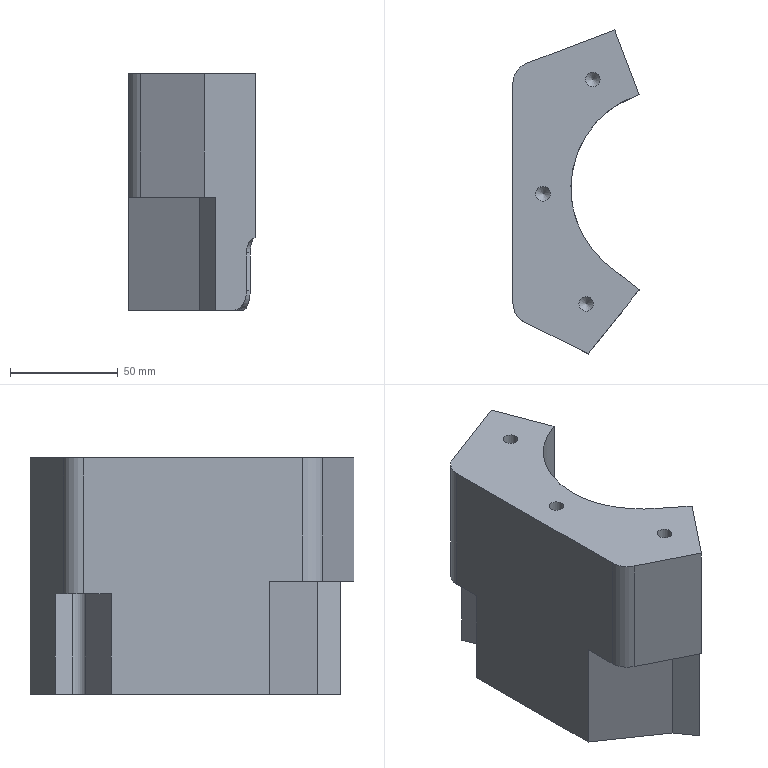Part | NX | features 8 2 | 1 solid | 38 faces | box 58.524 x 150.094 x 109.5 mm | volume 519516 mm3 | plane 15 | cylinder 13 | cone 5 | spline 4 | torus 1 | commonest cylinder face diameters 6.8 x3 8.5 x2 14 x2 18 x2 20 x2 10 x1
STEP:
#1=CARTESIAN_POINT('',(1901.4,-118.,66.));
#2=VERTEX_POINT('',#1);
#3=CARTESIAN_POINT('',(1898.,-118.,66.));
#4=DIRECTION('',(0.,0.,1.));
#5=DIRECTION('',(1.,0.,0.));
#6=AXIS2_PLACEMENT_3D('',#3,#4,#5);
#7=CIRCLE('',#6,3.4);
#8=EDGE_CURVE('',#2,#2,#7,.T.);
#9=ORIENTED_EDGE('',*,*,#8,.F.);
#10=EDGE_LOOP('',(#9));
#11=FACE_BOUND('',#10,.T.);
#12=CARTESIAN_POINT('',(1884.,-66.828,66.));
#13=VERTEX_POINT('',#12);
#14=CARTESIAN_POINT('',(1884.,-168.522,66.));
#15=VERTEX_POINT('',#14);
#16=CARTESIAN_POINT('',(1884.,-218.467,66.));
#17=DIRECTION('',(0.,-1.,0.));
#18=VECTOR('',#17,1000.);
#19=LINE('',#16,#18);
#20=EDGE_CURVE('',#13,#15,#19,.T.);
#21=ORIENTED_EDGE('',*,*,#20,.T.);
#22=CARTESIAN_POINT('',(1889.537,-177.471,66.));
#23=VERTEX_POINT('',#22);
#24=CARTESIAN_POINT('',(1894.,-168.522,66.));
#25=DIRECTION('',(0.,0.,1.));
#26=DIRECTION('',(1.,0.,0.));
#27=AXIS2_PLACEMENT_3D('',#24,#25,#26);
#28=CIRCLE('',#27,10.);
#29=EDGE_CURVE('',#15,#23,#28,.T.);
#30=ORIENTED_EDGE('',*,*,#29,.T.);
#31=CARTESIAN_POINT('',(1918.94,-192.136,66.));
#32=VERTEX_POINT('',#31);
#33=CARTESIAN_POINT('',(2033.826,-249.437,66.));
#34=DIRECTION('',(0.8949,-0.4463,0.));
#35=VECTOR('',#34,1000.);
#36=LINE('',#33,#35);
#37=EDGE_CURVE('',#23,#32,#36,.T.);
#38=ORIENTED_EDGE('',*,*,#37,.T.);
#39=CARTESIAN_POINT('',(1942.524,-162.487,66.));
#40=VERTEX_POINT('',#39);
#41=CARTESIAN_POINT('',(1956.62,-144.766,66.));
#42=DIRECTION('',(0.6225,0.7826,0.));
#43=VECTOR('',#42,1000.);
#44=LINE('',#41,#43);
#45=EDGE_CURVE('',#32,#40,#44,.T.);
#46=ORIENTED_EDGE('',*,*,#45,.T.);
#47=CARTESIAN_POINT('',(1942.524,-71.965,66.));
#48=VERTEX_POINT('',#47);
#49=CARTESIAN_POINT('',(1942.524,-71.965,66.));
#50=CARTESIAN_POINT('',(1940.246,-72.828,66.));
#51=CARTESIAN_POINT('',(1935.71,-74.591,66.));
#52=CARTESIAN_POINT('',(1929.54,-78.399,66.));
#53=CARTESIAN_POINT('',(1923.928,-83.204,66.));
#54=CARTESIAN_POINT('',(1919.28,-88.703,66.));
#55=CARTESIAN_POINT('',(1915.465,-95.025,66.));
#56=CARTESIAN_POINT('',(1912.762,-101.765,66.));
#57=CARTESIAN_POINT('',(1911.14,-108.951,66.));
#58=CARTESIAN_POINT('',(1910.547,-118.647,66.));
#59=CARTESIAN_POINT('',(1912.303,-128.367,66.));
#60=CARTESIAN_POINT('',(1916.274,-137.266,66.));
#61=CARTESIAN_POINT('',(1920.299,-143.399,66.));
#62=CARTESIAN_POINT('',(1925.194,-148.787,66.));
#63=CARTESIAN_POINT('',(1932.973,-154.837,66.));
#64=CARTESIAN_POINT('',(1938.688,-159.435,66.));
#65=CARTESIAN_POINT('',(1942.524,-162.487,66.));
#66=B_SPLINE_CURVE_WITH_KNOTS('',3,(#49,#50,#51,#52,#53,#54,#55,#56,#57,#58,#59,#60,#61,#62,#63,#64,#65),.UNSPECIFIED.,.F.,.F.,(4,1,1,1,1,1,1,1,1,1,1,1,1,1,4),(0.,0.007238,0.01448,0.02172,0.02895,0.03619,0.04343,0.05067,0.05791,0.07238,0.07962,0.08686,0.0941,0.1013,0.1158),.UNSPECIFIED.);
#67=EDGE_CURVE('',#48,#40,#66,.T.);
#68=ORIENTED_EDGE('',*,*,#67,.F.);
#69=CARTESIAN_POINT('',(1931.184,-42.042,66.));
#70=VERTEX_POINT('',#69);
#71=CARTESIAN_POINT('',(2004.479,-235.443,66.));
#72=DIRECTION('',(-0.3544,0.9351,0.));
#73=VECTOR('',#72,1000.);
#74=LINE('',#71,#73);
#75=EDGE_CURVE('',#48,#70,#74,.T.);
#76=ORIENTED_EDGE('',*,*,#75,.T.);
#77=CARTESIAN_POINT('',(1890.456,-57.477,66.));
#78=VERTEX_POINT('',#77);
#79=CARTESIAN_POINT('',(1990.095,-19.716,66.));
#80=DIRECTION('',(0.9351,0.3544,0.));
#81=VECTOR('',#80,1000.);
#82=LINE('',#79,#81);
#83=EDGE_CURVE('',#78,#70,#82,.T.);
#84=ORIENTED_EDGE('',*,*,#83,.F.);
#85=CARTESIAN_POINT('',(1894.,-66.828,66.));
#86=DIRECTION('',(0.,0.,1.));
#87=DIRECTION('',(1.,0.,0.));
#88=AXIS2_PLACEMENT_3D('',#85,#86,#87);
#89=CIRCLE('',#88,10.);
#90=EDGE_CURVE('',#78,#13,#89,.T.);
#91=ORIENTED_EDGE('',*,*,#90,.T.);
#92=EDGE_LOOP('',(#21,#30,#38,#46,#68,#76,#84,#91));
#93=FACE_BOUND('',#92,.T.);
#94=CARTESIAN_POINT('',(1921.4,-169.,66.));
#95=VERTEX_POINT('',#94);
#96=CARTESIAN_POINT('',(1918.,-169.,66.));
#97=DIRECTION('',(0.,0.,1.));
#98=DIRECTION('',(1.,0.,0.));
#99=AXIS2_PLACEMENT_3D('',#96,#97,#98);
#100=CIRCLE('',#99,3.4);
#101=EDGE_CURVE('',#95,#95,#100,.T.);
#102=ORIENTED_EDGE('',*,*,#101,.F.);
#103=EDGE_LOOP('',(#102));
#104=FACE_BOUND('',#103,.T.);
#105=CARTESIAN_POINT('',(1924.4,-65.,66.));
#106=VERTEX_POINT('',#105);
#107=CARTESIAN_POINT('',(1921.,-65.,66.));
#108=DIRECTION('',(0.,0.,1.));
#109=DIRECTION('',(1.,0.,0.));
#110=AXIS2_PLACEMENT_3D('',#107,#108,#109);
#111=CIRCLE('',#110,3.4);
#112=EDGE_CURVE('',#106,#106,#111,.T.);
#113=ORIENTED_EDGE('',*,*,#112,.F.);
#114=EDGE_LOOP('',(#113));
#115=FACE_BOUND('',#114,.T.);
#116=CARTESIAN_POINT('',(2049.273,-218.467,66.));
#117=DIRECTION('',(0.,0.,1.));
#118=DIRECTION('',(-1.,0.,0.));
#119=AXIS2_PLACEMENT_3D('',#116,#117,#118);
#120=PLANE('',#119);
#121=ADVANCED_FACE('',(#11,#93,#104,#115),#120,.T.);
#122=CARTESIAN_POINT('',(1884.,-79.693,3.));
#123=VERTEX_POINT('',#122);
#124=CARTESIAN_POINT('',(1884.,-66.828,3.));
#125=VERTEX_POINT('',#124);
#126=CARTESIAN_POINT('',(1884.,-36.,3.));
#127=DIRECTION('',(0.,1.,0.));
#128=VECTOR('',#127,1000.);
#129=LINE('',#126,#128);
#130=EDGE_CURVE('',#123,#125,#129,.T.);
#131=ORIENTED_EDGE('',*,*,#130,.T.);
#132=CARTESIAN_POINT('',(1890.456,-57.477,3.));
#133=VERTEX_POINT('',#132);
#134=CARTESIAN_POINT('',(1894.,-66.828,3.));
#135=DIRECTION('',(0.,0.,-1.));
#136=DIRECTION('',(1.,0.,0.));
#137=AXIS2_PLACEMENT_3D('',#134,#135,#136);
#138=CIRCLE('',#137,10.);
#139=EDGE_CURVE('',#125,#133,#138,.T.);
#140=ORIENTED_EDGE('',*,*,#139,.T.);
#141=CARTESIAN_POINT('',(1900.443,-53.692,3.));
#142=VERTEX_POINT('',#141);
#143=CARTESIAN_POINT('',(1990.095,-19.716,3.));
#144=DIRECTION('',(0.9351,0.3544,0.));
#145=VECTOR('',#144,1000.);
#146=LINE('',#143,#145);
#147=EDGE_CURVE('',#133,#142,#146,.T.);
#148=ORIENTED_EDGE('',*,*,#147,.T.);
#149=CARTESIAN_POINT('',(1903.559,-61.916,3.));
#150=VERTEX_POINT('',#149);
#151=CARTESIAN_POINT('',(1902.952,-60.314,3.));
#152=DIRECTION('',(-0.3544,0.9351,0.));
#153=VECTOR('',#152,1000.);
#154=LINE('',#151,#153);
#155=EDGE_CURVE('',#150,#142,#154,.T.);
#156=ORIENTED_EDGE('',*,*,#155,.F.);
#157=CARTESIAN_POINT('',(1901.669,-67.84,3.));
#158=VERTEX_POINT('',#157);
#159=CARTESIAN_POINT('',(1898.884,-63.688,3.));
#160=DIRECTION('',(0.,0.,-1.));
#161=DIRECTION('',(1.,0.,0.));
#162=AXIS2_PLACEMENT_3D('',#159,#160,#161);
#163=CIRCLE('',#162,5.);
#164=EDGE_CURVE('',#150,#158,#163,.T.);
#165=ORIENTED_EDGE('',*,*,#164,.T.);
#166=CARTESIAN_POINT('',(1894.226,-72.833,3.));
#167=DIRECTION('',(0.8305,0.5571,0.));
#168=VECTOR('',#167,1000.);
#169=LINE('',#166,#168);
#170=EDGE_CURVE('',#123,#158,#169,.T.);
#171=ORIENTED_EDGE('',*,*,#170,.F.);
#172=EDGE_LOOP('',(#131,#140,#148,#156,#165,#171));
#173=FACE_BOUND('',#172,.T.);
#174=CARTESIAN_POINT('',(1899.25,-66.,3.));
#175=VERTEX_POINT('',#174);
#176=CARTESIAN_POINT('',(1895.,-66.,3.));
#177=DIRECTION('',(0.,0.,-1.));
#178=DIRECTION('',(1.,0.,0.));
#179=AXIS2_PLACEMENT_3D('',#176,#177,#178);
#180=CIRCLE('',#179,4.25);
#181=EDGE_CURVE('',#175,#175,#180,.T.);
#182=ORIENTED_EDGE('',*,*,#181,.F.);
#183=EDGE_LOOP('',(#182));
#184=FACE_BOUND('',#183,.T.);
#185=CARTESIAN_POINT('',(1890.975,-67.988,3.));
#186=DIRECTION('',(0.,0.,1.));
#187=DIRECTION('',(-1.,0.,0.));
#188=AXIS2_PLACEMENT_3D('',#185,#186,#187);
#189=PLANE('',#188);
#190=ADVANCED_FACE('',(#173,#184),#189,.F.);
#191=CARTESIAN_POINT('',(1884.,-79.693,-43.5));
#192=VERTEX_POINT('',#191);
#193=CARTESIAN_POINT('',(1884.,-79.693,0.));
#194=DIRECTION('',(0.,0.,1.));
#195=VECTOR('',#194,1000.);
#196=LINE('',#193,#195);
#197=EDGE_CURVE('',#192,#123,#196,.T.);
#198=ORIENTED_EDGE('',*,*,#197,.F.);
#199=CARTESIAN_POINT('',(1884.,-152.801,-43.5));
#200=VERTEX_POINT('',#199);
#201=CARTESIAN_POINT('',(1884.,-66.746,-43.5));
#202=DIRECTION('',(0.,1.,0.000000004));
#203=VECTOR('',#202,1000.);
#204=LINE('',#201,#203);
#205=EDGE_CURVE('',#200,#192,#204,.T.);
#206=ORIENTED_EDGE('',*,*,#205,.F.);
#207=CARTESIAN_POINT('',(1884.,-152.801,8.9));
#208=VERTEX_POINT('',#207);
#209=CARTESIAN_POINT('',(1884.,-152.801,0.));
#210=DIRECTION('',(0.,0.,-1.));
#211=VECTOR('',#210,1000.);
#212=LINE('',#209,#211);
#213=EDGE_CURVE('',#208,#200,#212,.T.);
#214=ORIENTED_EDGE('',*,*,#213,.F.);
#215=CARTESIAN_POINT('',(1884.,-168.522,8.9));
#216=VERTEX_POINT('',#215);
#217=CARTESIAN_POINT('',(1884.,-36.,8.9));
#218=DIRECTION('',(0.,1.,0.));
#219=VECTOR('',#218,1000.);
#220=LINE('',#217,#219);
#221=EDGE_CURVE('',#216,#208,#220,.T.);
#222=ORIENTED_EDGE('',*,*,#221,.F.);
#223=CARTESIAN_POINT('',(1884.,-168.522,0.));
#224=DIRECTION('',(0.,0.,1.));
#225=VECTOR('',#224,1000.);
#226=LINE('',#223,#225);
#227=EDGE_CURVE('',#216,#15,#226,.T.);
#228=ORIENTED_EDGE('',*,*,#227,.T.);
#229=ORIENTED_EDGE('',*,*,#20,.F.);
#230=CARTESIAN_POINT('',(1884.,-66.828,0.));
#231=DIRECTION('',(0.,0.,-1.));
#232=VECTOR('',#231,1000.);
#233=LINE('',#230,#232);
#234=EDGE_CURVE('',#13,#125,#233,.T.);
#235=ORIENTED_EDGE('',*,*,#234,.T.);
#236=ORIENTED_EDGE('',*,*,#130,.F.);
#237=EDGE_LOOP('',(#198,#206,#214,#222,#228,#229,#235,#236));
#238=FACE_BOUND('',#237,.T.);
#239=CARTESIAN_POINT('',(1884.,-36.,0.));
#240=DIRECTION('',(-1.,0.,0.));
#241=DIRECTION('',(0.,0.,-1.));
#242=AXIS2_PLACEMENT_3D('',#239,#240,#241);
#243=PLANE('',#242);
#244=ADVANCED_FACE('',(#238),#243,.T.);
#245=ORIENTED_EDGE('',*,*,#37,.F.);
#246=CARTESIAN_POINT('',(1889.537,-177.471,8.9));
#247=VERTEX_POINT('',#246);
#248=CARTESIAN_POINT('',(1889.537,-177.471,-27.5));
#249=DIRECTION('',(0.,0.,-1.));
#250=VECTOR('',#249,1000.);
#251=LINE('',#248,#250);
#252=EDGE_CURVE('',#23,#247,#251,.T.);
#253=ORIENTED_EDGE('',*,*,#252,.T.);
#254=CARTESIAN_POINT('',(1918.94,-192.136,8.9));
#255=VERTEX_POINT('',#254);
#256=CARTESIAN_POINT('',(1975.42,-220.307,8.9));
#257=DIRECTION('',(-0.8949,0.4463,0.));
#258=VECTOR('',#257,1000.);
#259=LINE('',#256,#258);
#260=EDGE_CURVE('',#255,#247,#259,.T.);
#261=ORIENTED_EDGE('',*,*,#260,.F.);
#262=CARTESIAN_POINT('',(1918.94,-192.136,-116.522));
#263=DIRECTION('',(0.,0.,-1.));
#264=VECTOR('',#263,1000.);
#265=LINE('',#262,#264);
#266=EDGE_CURVE('',#32,#255,#265,.T.);
#267=ORIENTED_EDGE('',*,*,#266,.F.);
#268=EDGE_LOOP('',(#245,#253,#261,#267));
#269=FACE_BOUND('',#268,.T.);
#270=CARTESIAN_POINT('',(1975.42,-220.307,-27.5));
#271=DIRECTION('',(-0.4463,-0.8949,0.));
#272=DIRECTION('',(-0.8949,0.4463,0.));
#273=AXIS2_PLACEMENT_3D('',#270,#271,#272);
#274=PLANE('',#273);
#275=ADVANCED_FACE('',(#269),#274,.T.);
#276=CARTESIAN_POINT('',(1924.001,-185.773,8.9));
#277=VERTEX_POINT('',#276);
#278=CARTESIAN_POINT('',(1885.875,-233.704,8.9));
#279=DIRECTION('',(-0.6225,-0.7826,0.));
#280=VECTOR('',#279,1000.);
#281=LINE('',#278,#280);
#282=EDGE_CURVE('',#277,#255,#281,.T.);
#283=ORIENTED_EDGE('',*,*,#282,.F.);
#284=CARTESIAN_POINT('',(1924.001,-185.773,-43.5));
#285=VERTEX_POINT('',#284);
#286=CARTESIAN_POINT('',(1924.001,-185.773,-116.522));
#287=DIRECTION('',(0.,0.,-1.));
#288=VECTOR('',#287,1000.);
#289=LINE('',#286,#288);
#290=EDGE_CURVE('',#277,#285,#289,.T.);
#291=ORIENTED_EDGE('',*,*,#290,.T.);
#292=CARTESIAN_POINT('',(1932.875,-174.617,-43.5));
#293=VERTEX_POINT('',#292);
#294=CARTESIAN_POINT('',(1938.478,-167.574,-43.5));
#295=DIRECTION('',(-0.6225,-0.7826,-0.000000003));
#296=VECTOR('',#295,1000.);
#297=LINE('',#294,#296);
#298=EDGE_CURVE('',#293,#285,#297,.T.);
#299=ORIENTED_EDGE('',*,*,#298,.F.);
#300=CARTESIAN_POINT('',(1938.478,-167.574,-34.5));
#301=VERTEX_POINT('',#300);
#302=CARTESIAN_POINT('',(1932.875,-174.617,-34.5));
#303=DIRECTION('',(0.7826,-0.6225,0.));
#304=DIRECTION('',(0.6225,0.7826,0.));
#305=AXIS2_PLACEMENT_3D('',#302,#303,#304);
#306=CIRCLE('',#305,9.);
#307=EDGE_CURVE('',#293,#301,#306,.T.);
#308=ORIENTED_EDGE('',*,*,#307,.T.);
#309=CARTESIAN_POINT('',(1938.478,-167.574,-17.));
#310=VERTEX_POINT('',#309);
#311=CARTESIAN_POINT('',(1938.478,-167.574,-0.00000039));
#312=DIRECTION('',(-0.000000002,-0.000000002,1.));
#313=VECTOR('',#312,1000.);
#314=LINE('',#311,#313);
#315=EDGE_CURVE('',#301,#310,#314,.T.);
#316=ORIENTED_EDGE('',*,*,#315,.T.);
#317=CARTESIAN_POINT('',(1942.524,-162.487,-10.018));
#318=VERTEX_POINT('',#317);
#319=CARTESIAN_POINT('',(1942.835,-162.095,-17.));
#320=DIRECTION('',(-0.7826,0.6225,0.));
#321=DIRECTION('',(0.6225,0.7826,0.));
#322=AXIS2_PLACEMENT_3D('',#319,#320,#321);
#323=CIRCLE('',#322,7.);
#324=EDGE_CURVE('',#310,#318,#323,.T.);
#325=ORIENTED_EDGE('',*,*,#324,.T.);
#326=CARTESIAN_POINT('',(1942.524,-162.487,7.385));
#327=DIRECTION('',(0.,0.,-1.));
#328=VECTOR('',#327,1000.);
#329=LINE('',#326,#328);
#330=EDGE_CURVE('',#40,#318,#329,.T.);
#331=ORIENTED_EDGE('',*,*,#330,.F.);
#332=ORIENTED_EDGE('',*,*,#45,.F.);
#333=ORIENTED_EDGE('',*,*,#266,.T.);
#334=EDGE_LOOP('',(#283,#291,#299,#308,#316,#325,#331,#332,#333));
#335=FACE_BOUND('',#334,.T.);
#336=CARTESIAN_POINT('',(1885.875,-233.704,-116.522));
#337=DIRECTION('',(0.7826,-0.6225,0.));
#338=DIRECTION('',(-0.6225,-0.7826,0.));
#339=AXIS2_PLACEMENT_3D('',#336,#337,#338);
#340=PLANE('',#339);
#341=ADVANCED_FACE('',(#335),#340,.T.);
#342=ORIENTED_EDGE('',*,*,#298,.T.);
#343=CARTESIAN_POINT('',(1916.658,-175.233,-43.5));
#344=VERTEX_POINT('',#343);
#345=CARTESIAN_POINT('',(1872.732,-112.188,-43.5));
#346=DIRECTION('',(-0.5717,0.8205,0.000000004));
#347=VECTOR('',#346,1000.);
#348=LINE('',#345,#347);
#349=EDGE_CURVE('',#285,#344,#348,.T.);
#350=ORIENTED_EDGE('',*,*,#349,.T.);
#351=CARTESIAN_POINT('',(1880.497,-150.395,-43.5));
#352=DIRECTION('',(0.8243,-0.5662,-0.000000003));
#353=VECTOR('',#352,1000.);
#354=LINE('',#351,#353);
#355=EDGE_CURVE('',#200,#344,#354,.T.);
#356=ORIENTED_EDGE('',*,*,#355,.F.);
#357=ORIENTED_EDGE('',*,*,#205,.T.);
#358=CARTESIAN_POINT('',(1901.669,-67.84,-43.5));
#359=VERTEX_POINT('',#358);
#360=CARTESIAN_POINT('',(1927.2,-50.714,-43.5));
#361=DIRECTION('',(-0.8305,-0.5571,-0.000000002));
#362=VECTOR('',#361,1000.);
#363=LINE('',#360,#362);
#364=EDGE_CURVE('',#359,#192,#363,.T.);
#365=ORIENTED_EDGE('',*,*,#364,.F.);
#366=CARTESIAN_POINT('',(1903.559,-61.916,-43.5));
#367=VERTEX_POINT('',#366);
#368=CARTESIAN_POINT('',(1898.884,-63.688,-43.5));
#369=DIRECTION('',(0.000000001,-0.000000004,1.));
#370=DIRECTION('',(0.,1.,0.000000004));
#371=AXIS2_PLACEMENT_3D('',#368,#369,#370);
#372=CIRCLE('',#371,5.);
#373=EDGE_CURVE('',#359,#367,#372,.T.);
#374=ORIENTED_EDGE('',*,*,#373,.T.);
#375=CARTESIAN_POINT('',(1900.443,-53.692,-43.5));
#376=VERTEX_POINT('',#375);
#377=CARTESIAN_POINT('',(1909.48,-77.537,-43.5));
#378=DIRECTION('',(0.3544,-0.9351,-0.000000004));
#379=VECTOR('',#378,1000.);
#380=LINE('',#377,#379);
#381=EDGE_CURVE('',#376,#367,#380,.T.);
#382=ORIENTED_EDGE('',*,*,#381,.F.);
#383=CARTESIAN_POINT('',(1931.184,-42.042,-43.5));
#384=VERTEX_POINT('',#383);
#385=CARTESIAN_POINT('',(1990.095,-19.716,-43.5));
#386=DIRECTION('',(-0.9351,-0.3544,-0.000000001));
#387=VECTOR('',#386,1000.);
#388=LINE('',#385,#387);
#389=EDGE_CURVE('',#384,#376,#388,.T.);
#390=ORIENTED_EDGE('',*,*,#389,.F.);
#391=CARTESIAN_POINT('',(1937.031,-57.471,-43.5));
#392=VERTEX_POINT('',#391);
#393=CARTESIAN_POINT('',(1940.221,-65.887,-43.5));
#394=DIRECTION('',(-0.3544,0.9351,0.000000004));
#395=VECTOR('',#394,1000.);
#396=LINE('',#393,#395);
#397=EDGE_CURVE('',#392,#384,#396,.T.);
#398=ORIENTED_EDGE('',*,*,#397,.F.);
#399=CARTESIAN_POINT('',(1934.761,-58.331,-43.5));
#400=VERTEX_POINT('',#399);
#401=CARTESIAN_POINT('',(1937.031,-57.471,-43.5));
#402=CARTESIAN_POINT('',(1936.275,-57.758,-43.5));
#403=CARTESIAN_POINT('',(1935.518,-58.045,-43.5));
#404=CARTESIAN_POINT('',(1934.761,-58.331,-43.5));
#405=B_SPLINE_CURVE_WITH_KNOTS('',3,(#401,#402,#403,#404),.UNSPECIFIED.,.F.,.F.,(4,4),(0.,1.),.PIECEWISE_BEZIER_KNOTS.);
#406=EDGE_CURVE('',#392,#400,#405,.T.);
#407=ORIENTED_EDGE('',*,*,#406,.T.);
#408=CARTESIAN_POINT('',(1918.407,-163.108,-43.5));
#409=VERTEX_POINT('',#408);
#410=CARTESIAN_POINT('',(1934.761,-58.331,-43.5));
#411=CARTESIAN_POINT('',(1933.539,-58.796,-43.5));
#412=CARTESIAN_POINT('',(1931.034,-59.837,-43.5));
#413=CARTESIAN_POINT('',(1926.249,-62.216,-43.5));
#414=CARTESIAN_POINT('',(1918.279,-67.207,-43.5));
#415=CARTESIAN_POINT('',(1908.459,-76.481,-43.5));
#416=CARTESIAN_POINT('',(1900.024,-90.316,-43.5));
#417=CARTESIAN_POINT('',(1895.397,-105.855,-43.5));
#418=CARTESIAN_POINT('',(1895.063,-122.038,-43.5));
#419=CARTESIAN_POINT('',(1898.885,-137.806,-43.5));
#420=CARTESIAN_POINT('',(1905.421,-149.636,-43.5));
#421=CARTESIAN_POINT('',(1911.469,-156.801,-43.5));
#422=CARTESIAN_POINT('',(1915.332,-160.551,-43.5));
#423=CARTESIAN_POINT('',(1917.34,-162.258,-43.5));
#424=CARTESIAN_POINT('',(1918.407,-163.108,-43.5));
#425=B_SPLINE_CURVE_WITH_KNOTS('',3,(#410,#411,#412,#413,#414,#415,#416,#417,#418,#419,#420,#421,#422,#423,#424),.UNSPECIFIED.,.F.,.F.,(4,1,1,1,1,1,1,1,1,1,1,1,4),(0.,0.03125,0.0625,0.125,0.25,0.375,0.5,0.625,0.75,0.875,0.9375,0.9688,1.),.UNSPECIFIED.);
#426=EDGE_CURVE('',#400,#409,#425,.T.);
#427=ORIENTED_EDGE('',*,*,#426,.T.);
#428=CARTESIAN_POINT('',(1918.407,-163.108,-43.5));
#429=CARTESIAN_POINT('',(1923.229,-166.944,-43.5));
#430=CARTESIAN_POINT('',(1928.052,-170.781,-43.5));
#431=CARTESIAN_POINT('',(1932.875,-174.617,-43.5));
#432=B_SPLINE_CURVE_WITH_KNOTS('',3,(#428,#429,#430,#431),.UNSPECIFIED.,.F.,.F.,(4,4),(0.,1.),.PIECEWISE_BEZIER_KNOTS.);
#433=EDGE_CURVE('',#409,#293,#432,.T.);
#434=ORIENTED_EDGE('',*,*,#433,.T.);
#435=EDGE_LOOP('',(#342,#350,#356,#357,#365,#374,#382,#390,#398,#407,#427,#434));
#436=FACE_BOUND('',#435,.T.);
#437=CARTESIAN_POINT('',(1937.954,-66.746,-43.5));
#438=DIRECTION('',(-0.000000001,0.000000004,-1.));
#439=DIRECTION('',(0.3552,-0.9348,-0.000000004));
#440=AXIS2_PLACEMENT_3D('',#437,#438,#439);
#441=PLANE('',#440);
#442=ADVANCED_FACE('',(#436),#441,.T.);
#443=CARTESIAN_POINT('',(1940.221,-65.887,-34.5));
#444=VERTEX_POINT('',#443);
#445=CARTESIAN_POINT('',(1937.031,-57.471,-34.5));
#446=DIRECTION('',(0.9351,0.3544,0.));
#447=DIRECTION('',(-0.3544,0.9351,0.));
#448=AXIS2_PLACEMENT_3D('',#445,#446,#447);
#449=CIRCLE('',#448,9.);
#450=EDGE_CURVE('',#444,#392,#449,.T.);
#451=ORIENTED_EDGE('',*,*,#450,.F.);
#452=CARTESIAN_POINT('',(1937.954,-66.746,-34.5));
#453=VERTEX_POINT('',#452);
#454=CARTESIAN_POINT('',(1959.053,-58.75,-34.5));
#455=DIRECTION('',(-0.9351,-0.3544,-0.000000001));
#456=VECTOR('',#455,1000.);
#457=LINE('',#454,#456);
#458=EDGE_CURVE('',#444,#453,#457,.T.);
#459=ORIENTED_EDGE('',*,*,#458,.T.);
#460=CARTESIAN_POINT('',(1934.765,-58.33,-34.5));
#461=DIRECTION('',(-0.9351,-0.3544,-0.000000001));
#462=DIRECTION('',(-0.3544,0.9351,0.000000003));
#463=AXIS2_PLACEMENT_3D('',#460,#461,#462);
#464=CIRCLE('',#463,9.);
#465=EDGE_CURVE('',#400,#453,#464,.T.);
#466=ORIENTED_EDGE('',*,*,#465,.F.);
#467=ORIENTED_EDGE('',*,*,#406,.F.);
#468=EDGE_LOOP('',(#451,#459,#466,#467));
#469=FACE_BOUND('',#468,.T.);
#470=CARTESIAN_POINT('',(1977.312,-42.205,-34.5));
#471=DIRECTION('',(-0.9351,-0.3544,-0.000000001));
#472=DIRECTION('',(-0.3544,0.9351,0.));
#473=AXIS2_PLACEMENT_3D('',#470,#471,#472);
#474=CYLINDRICAL_SURFACE('',#473,9.);
#475=ADVANCED_FACE('',(#469),#474,.T.);
#476=CARTESIAN_POINT('',(1940.221,-65.887,-17.));
#477=VERTEX_POINT('',#476);
#478=CARTESIAN_POINT('',(1940.221,-65.887,0.000000056));
#479=DIRECTION('',(-0.000000001,0.000000004,-1.));
#480=VECTOR('',#479,1000.);
#481=LINE('',#478,#480);
#482=EDGE_CURVE('',#477,#444,#481,.T.);
#483=ORIENTED_EDGE('',*,*,#482,.F.);
#484=CARTESIAN_POINT('',(1937.954,-66.746,-17.));
#485=VERTEX_POINT('',#484);
#486=CARTESIAN_POINT('',(1960.935,-58.037,-17.));
#487=DIRECTION('',(-0.9351,-0.3544,-0.000000001));
#488=VECTOR('',#487,1000.);
#489=LINE('',#486,#488);
#490=EDGE_CURVE('',#477,#485,#489,.T.);
#491=ORIENTED_EDGE('',*,*,#490,.T.);
#492=CARTESIAN_POINT('',(1937.954,-66.746,-22.75));
#493=DIRECTION('',(0.000000001,-0.000000004,1.));
#494=VECTOR('',#493,1000.);
#495=LINE('',#492,#494);
#496=EDGE_CURVE('',#453,#485,#495,.T.);
#497=ORIENTED_EDGE('',*,*,#496,.F.);
#498=ORIENTED_EDGE('',*,*,#458,.F.);
#499=EDGE_LOOP('',(#483,#491,#497,#498));
#500=FACE_BOUND('',#499,.T.);
#501=CARTESIAN_POINT('',(2038.436,-28.665,0.000000056));
#502=DIRECTION('',(-0.3544,0.9351,0.000000004));
#503=DIRECTION('',(0.9351,0.3544,0.000000001));
#504=AXIS2_PLACEMENT_3D('',#501,#502,#503);
#505=PLANE('',#504);
#506=ADVANCED_FACE('',(#500),#505,.F.);
#507=CARTESIAN_POINT('',(1937.948,-66.748,-34.5));
#508=VERTEX_POINT('',#507);
#509=CARTESIAN_POINT('',(1937.948,-66.748,-34.5));
#510=CARTESIAN_POINT('',(1937.948,-66.748,-35.561));
#511=CARTESIAN_POINT('',(1937.812,-66.389,-37.852));
#512=CARTESIAN_POINT('',(1937.081,-64.461,-41.054));
#513=CARTESIAN_POINT('',(1935.946,-61.467,-43.116));
#514=CARTESIAN_POINT('',(1935.133,-59.325,-43.5));
#515=CARTESIAN_POINT('',(1934.757,-58.333,-43.5));
#516=B_SPLINE_CURVE_WITH_KNOTS('',3,(#509,#510,#511,#512,#513,#514,#515),.UNSPECIFIED.,.F.,.F.,(4,1,1,1,4),(0.,0.25,0.5,0.75,1.),.UNSPECIFIED.);
#517=EDGE_CURVE('',#400,#508,#516,.F.);
#518=ORIENTED_EDGE('',*,*,#517,.F.);
#519=ORIENTED_EDGE('',*,*,#465,.T.);
#520=CARTESIAN_POINT('',(1937.954,-66.746,-34.5));
#521=CARTESIAN_POINT('',(1937.952,-66.747,-34.5));
#522=CARTESIAN_POINT('',(1937.95,-66.747,-34.5));
#523=CARTESIAN_POINT('',(1937.948,-66.748,-34.5));
#524=B_SPLINE_CURVE_WITH_KNOTS('',3,(#520,#521,#522,#523),.UNSPECIFIED.,.F.,.F.,(4,4),(0.,1.),.PIECEWISE_BEZIER_KNOTS.);
#525=EDGE_CURVE('',#453,#508,#524,.T.);
#526=ORIENTED_EDGE('',*,*,#525,.T.);
#527=EDGE_LOOP('',(#518,#519,#526));
#528=FACE_BOUND('',#527,.T.);
#529=CARTESIAN_POINT('',(1934.765,-58.33,-43.5));
#530=CARTESIAN_POINT('',(1937.954,-66.746,-43.5));
#531=CARTESIAN_POINT('',(1937.954,-66.746,-34.5));
#532=CARTESIAN_POINT('',(1934.762,-58.331,-43.5));
#533=CARTESIAN_POINT('',(1937.952,-66.747,-43.5));
#534=CARTESIAN_POINT('',(1937.952,-66.747,-34.5));
#535=CARTESIAN_POINT('',(1934.76,-58.332,-43.5));
#536=CARTESIAN_POINT('',(1937.95,-66.747,-43.5));
#537=CARTESIAN_POINT('',(1937.95,-66.747,-34.5));
#538=CARTESIAN_POINT('',(1934.757,-58.333,-43.5));
#539=CARTESIAN_POINT('',(1937.948,-66.748,-43.5));
#540=CARTESIAN_POINT('',(1937.948,-66.748,-34.5));
#541=(BOUNDED_SURFACE()B_SPLINE_SURFACE(3,2,((#529,#530,#531),(#532,#533,#534),(#535,#536,#537),(#538,#539,#540)),.UNSPECIFIED.,.F.,.F.,.F.)B_SPLINE_SURFACE_WITH_KNOTS((4,4),(3,3),(0.,1.),(0.,1.),.PIECEWISE_BEZIER_KNOTS.)GEOMETRIC_REPRESENTATION_ITEM()RATIONAL_B_SPLINE_SURFACE(((1.,0.7071,1.),(1.,0.7071,1.),(1.,0.7071,1.),(1.,0.7071,1.)))REPRESENTATION_ITEM('')SURFACE());
#542=ADVANCED_FACE('',(#528),#541,.F.);
#543=ORIENTED_EDGE('',*,*,#426,.F.);
#544=ORIENTED_EDGE('',*,*,#517,.T.);
#545=CARTESIAN_POINT('',(1924.008,-156.063,-34.5));
#546=VERTEX_POINT('',#545);
#547=CARTESIAN_POINT('',(1924.008,-156.063,-34.5));
#548=CARTESIAN_POINT('',(1916.862,-150.378,-34.5));
#549=CARTESIAN_POINT('',(1905.647,-135.165,-34.5));
#550=CARTESIAN_POINT('',(1902.572,-106.972,-34.5));
#551=CARTESIAN_POINT('',(1914.092,-81.057,-34.5));
#552=CARTESIAN_POINT('',(1929.41,-69.985,-34.5));
#553=CARTESIAN_POINT('',(1937.948,-66.748,-34.5));
#554=B_SPLINE_CURVE_WITH_KNOTS('',3,(#547,#548,#549,#550,#551,#552,#553),.UNSPECIFIED.,.F.,.F.,(4,1,1,1,4),(0.,0.25,0.5,0.75,1.),.UNSPECIFIED.);
#555=EDGE_CURVE('',#508,#546,#554,.F.);
#556=ORIENTED_EDGE('',*,*,#555,.T.);
#557=CARTESIAN_POINT('',(1924.008,-156.063,-34.5));
#558=CARTESIAN_POINT('',(1924.008,-156.063,-35.561));
#559=CARTESIAN_POINT('',(1923.769,-156.363,-37.851));
#560=CARTESIAN_POINT('',(1922.488,-157.973,-41.051));
#561=CARTESIAN_POINT('',(1920.496,-160.477,-43.114));
#562=CARTESIAN_POINT('',(1919.067,-162.274,-43.5));
#563=CARTESIAN_POINT('',(1918.404,-163.106,-43.5));
#564=B_SPLINE_CURVE_WITH_KNOTS('',3,(#557,#558,#559,#560,#561,#562,#563),.UNSPECIFIED.,.F.,.F.,(4,1,1,1,4),(0.,0.25,0.5,0.75,1.),.UNSPECIFIED.);
#565=EDGE_CURVE('',#409,#546,#564,.F.);
#566=ORIENTED_EDGE('',*,*,#565,.F.);
#567=EDGE_LOOP('',(#543,#544,#556,#566));
#568=FACE_BOUND('',#567,.T.);
#569=CARTESIAN_POINT('',(1935.46,-57.984,-43.5));
#570=CARTESIAN_POINT('',(1935.473,-58.02,-43.5));
#571=CARTESIAN_POINT('',(1938.569,-66.513,-43.5));
#572=CARTESIAN_POINT('',(1938.569,-66.513,-34.5));
#573=CARTESIAN_POINT('',(1935.217,-58.076,-43.5));
#574=CARTESIAN_POINT('',(1935.23,-58.112,-43.5));
#575=CARTESIAN_POINT('',(1938.362,-66.591,-43.5));
#576=CARTESIAN_POINT('',(1938.362,-66.591,-34.5));
#577=CARTESIAN_POINT('',(1934.973,-58.168,-43.5));
#578=CARTESIAN_POINT('',(1934.987,-58.204,-43.5));
#579=CARTESIAN_POINT('',(1938.155,-66.67,-43.5));
#580=CARTESIAN_POINT('',(1938.155,-66.67,-34.5));
#581=CARTESIAN_POINT('',(1929.687,-60.172,-43.5));
#582=CARTESIAN_POINT('',(1929.704,-60.207,-43.5));
#583=CARTESIAN_POINT('',(1933.655,-68.376,-43.5));
#584=CARTESIAN_POINT('',(1933.655,-68.376,-34.5));
#585=CARTESIAN_POINT('',(1924.922,-62.748,-43.5));
#586=CARTESIAN_POINT('',(1924.942,-62.782,-43.5));
#587=CARTESIAN_POINT('',(1929.598,-70.569,-43.5));
#588=CARTESIAN_POINT('',(1929.598,-70.569,-34.5));
#589=CARTESIAN_POINT('',(1918.435,-67.438,-43.5));
#590=CARTESIAN_POINT('',(1918.459,-67.469,-43.5));
#591=CARTESIAN_POINT('',(1924.075,-74.562,-43.5));
#592=CARTESIAN_POINT('',(1924.075,-74.562,-34.5));
#593=CARTESIAN_POINT('',(1916.373,-69.144,-43.5));
#594=CARTESIAN_POINT('',(1916.398,-69.173,-43.5));
#595=CARTESIAN_POINT('',(1922.319,-76.014,-43.5));
#596=CARTESIAN_POINT('',(1922.319,-76.014,-34.5));
#597=CARTESIAN_POINT('',(1912.456,-72.849,-43.5));
#598=CARTESIAN_POINT('',(1912.483,-72.876,-43.5));
#599=CARTESIAN_POINT('',(1918.984,-79.169,-43.5));
#600=CARTESIAN_POINT('',(1918.984,-79.169,-34.5));
#601=CARTESIAN_POINT('',(1910.617,-74.835,-43.5));
#602=CARTESIAN_POINT('',(1910.646,-74.861,-43.5));
#603=CARTESIAN_POINT('',(1917.419,-80.86,-43.5));
#604=CARTESIAN_POINT('',(1917.419,-80.86,-34.5));
#605=CARTESIAN_POINT('',(1907.251,-78.989,-43.5));
#606=CARTESIAN_POINT('',(1907.282,-79.012,-43.5));
#607=CARTESIAN_POINT('',(1914.553,-84.396,-43.5));
#608=CARTESIAN_POINT('',(1914.553,-84.396,-34.5));
#609=CARTESIAN_POINT('',(1905.71,-81.167,-43.5));
#610=CARTESIAN_POINT('',(1905.742,-81.189,-43.5));
#611=CARTESIAN_POINT('',(1913.241,-86.25,-43.5));
#612=CARTESIAN_POINT('',(1913.241,-86.25,-34.5));
#613=CARTESIAN_POINT('',(1902.914,-85.727,-43.5));
#614=CARTESIAN_POINT('',(1902.948,-85.746,-43.5));
#615=CARTESIAN_POINT('',(1910.861,-90.133,-43.5));
#616=CARTESIAN_POINT('',(1910.861,-90.133,-34.5));
#617=CARTESIAN_POINT('',(1901.652,-88.127,-43.5));
#618=CARTESIAN_POINT('',(1901.686,-88.144,-43.5));
#619=CARTESIAN_POINT('',(1909.786,-92.176,-43.5));
#620=CARTESIAN_POINT('',(1909.786,-92.176,-34.5));
#621=CARTESIAN_POINT('',(1898.374,-95.511,-43.5));
#622=CARTESIAN_POINT('',(1898.41,-95.523,-43.5));
#623=CARTESIAN_POINT('',(1906.995,-98.463,-43.5));
#624=CARTESIAN_POINT('',(1906.995,-98.463,-34.5));
#625=CARTESIAN_POINT('',(1896.867,-100.63,-43.5));
#626=CARTESIAN_POINT('',(1896.905,-100.639,-43.5));
#627=CARTESIAN_POINT('',(1905.712,-102.821,-43.5));
#628=CARTESIAN_POINT('',(1905.712,-102.821,-34.5));
#629=CARTESIAN_POINT('',(1895.622,-108.603,-43.5));
#630=CARTESIAN_POINT('',(1895.66,-108.607,-43.5));
#631=CARTESIAN_POINT('',(1904.652,-109.609,-43.5));
#632=CARTESIAN_POINT('',(1904.652,-109.609,-34.5));
#633=CARTESIAN_POINT('',(1895.382,-111.308,-43.5));
#634=CARTESIAN_POINT('',(1895.42,-111.311,-43.5));
#635=CARTESIAN_POINT('',(1904.448,-111.912,-43.5));
#636=CARTESIAN_POINT('',(1904.448,-111.912,-34.5));
#637=CARTESIAN_POINT('',(1895.26,-116.66,-43.5));
#638=CARTESIAN_POINT('',(1895.299,-116.659,-43.5));
#639=CARTESIAN_POINT('',(1904.344,-116.468,-43.5));
#640=CARTESIAN_POINT('',(1904.344,-116.468,-34.5));
#641=CARTESIAN_POINT('',(1895.375,-119.325,-43.5));
#642=CARTESIAN_POINT('',(1895.413,-119.323,-43.5));
#643=CARTESIAN_POINT('',(1904.442,-118.738,-43.5));
#644=CARTESIAN_POINT('',(1904.442,-118.738,-34.5));
#645=CARTESIAN_POINT('',(1896.242,-127.294,-43.5));
#646=CARTESIAN_POINT('',(1896.28,-127.287,-43.5));
#647=CARTESIAN_POINT('',(1905.18,-125.522,-43.5));
#648=CARTESIAN_POINT('',(1905.18,-125.522,-34.5));
#649=CARTESIAN_POINT('',(1897.545,-132.606,-43.5));
#650=CARTESIAN_POINT('',(1897.582,-132.596,-43.5));
#651=CARTESIAN_POINT('',(1906.289,-130.045,-43.5));
#652=CARTESIAN_POINT('',(1906.289,-130.045,-34.5));
#653=CARTESIAN_POINT('',(1900.456,-140.065,-43.5));
#654=CARTESIAN_POINT('',(1900.491,-140.049,-43.5));
#655=CARTESIAN_POINT('',(1908.768,-136.395,-43.5));
#656=CARTESIAN_POINT('',(1908.768,-136.395,-34.5));
#657=CARTESIAN_POINT('',(1901.587,-142.484,-43.5));
#658=CARTESIAN_POINT('',(1901.622,-142.467,-43.5));
#659=CARTESIAN_POINT('',(1909.731,-138.455,-43.5));
#660=CARTESIAN_POINT('',(1909.731,-138.455,-34.5));
#661=CARTESIAN_POINT('',(1904.177,-147.187,-43.5));
#662=CARTESIAN_POINT('',(1904.21,-147.167,-43.5));
#663=CARTESIAN_POINT('',(1911.936,-142.459,-43.5));
#664=CARTESIAN_POINT('',(1911.936,-142.459,-34.5));
#665=CARTESIAN_POINT('',(1905.645,-149.478,-43.5));
#666=CARTESIAN_POINT('',(1905.677,-149.457,-43.5));
#667=CARTESIAN_POINT('',(1913.185,-144.409,-43.5));
#668=CARTESIAN_POINT('',(1913.185,-144.409,-34.5));
#669=CARTESIAN_POINT('',(1910.419,-155.948,-43.5));
#670=CARTESIAN_POINT('',(1910.448,-155.922,-43.5));
#671=CARTESIAN_POINT('',(1917.25,-149.917,-43.5));
#672=CARTESIAN_POINT('',(1917.25,-149.917,-34.5));
#673=CARTESIAN_POINT('',(1914.121,-159.797,-43.5));
#674=CARTESIAN_POINT('',(1914.147,-159.769,-43.5));
#675=CARTESIAN_POINT('',(1920.402,-153.194,-43.5));
#676=CARTESIAN_POINT('',(1920.402,-153.194,-34.5));
#677=CARTESIAN_POINT('',(1918.56,-163.329,-43.5));
#678=CARTESIAN_POINT('',(1918.584,-163.299,-43.5));
#679=CARTESIAN_POINT('',(1924.181,-156.202,-43.5));
#680=CARTESIAN_POINT('',(1924.181,-156.202,-34.5));
#681=CARTESIAN_POINT('',(1918.764,-163.491,-43.5));
#682=CARTESIAN_POINT('',(1918.788,-163.461,-43.5));
#683=CARTESIAN_POINT('',(1924.355,-156.34,-43.5));
#684=CARTESIAN_POINT('',(1924.355,-156.34,-34.5));
#685=CARTESIAN_POINT('',(1918.968,-163.654,-43.5));
#686=CARTESIAN_POINT('',(1918.992,-163.623,-43.5));
#687=CARTESIAN_POINT('',(1924.529,-156.478,-43.5));
#688=CARTESIAN_POINT('',(1924.529,-156.478,-34.5));
#689=(BOUNDED_SURFACE()B_SPLINE_SURFACE(3,2,((#569,#570,#571,#572),(#573,#574,#575,#576),(#577,#578,#579,#580),(#581,#582,#583,#584),(#585,#586,#587,#588),(#589,#590,#591,#592),(#593,#594,#595,#596),(#597,#598,#599,#600),(#601,#602,#603,#604),(#605,#606,#607,#608),(#609,#610,#611,#612),(#613,#614,#615,#616),(#617,#618,#619,#620),(#621,#622,#623,#624),(#625,#626,#627,#628),(#629,#630,#631,#632),(#633,#634,#635,#636),(#637,#638,#639,#640),(#641,#642,#643,#644),(#645,#646,#647,#648),(#649,#650,#651,#652),(#653,#654,#655,#656),(#657,#658,#659,#660),(#661,#662,#663,#664),(#665,#666,#667,#668),(#669,#670,#671,#672),(#673,#674,#675,#676),(#677,#678,#679,#680),(#681,#682,#683,#684),(#685,#686,#687,#688)),.UNSPECIFIED.,.F.,.F.,.F.)B_SPLINE_SURFACE_WITH_KNOTS((4,2,2,2,2,2,2,2,2,2,2,2,2,2,4),(3,1,3),(0.00389,0.009804,0.1324,0.1936,0.2549,0.3162,0.3775,0.5,0.5613,0.6225,0.7451,0.8064,0.8676,0.9902,0.9961),(0.003892,0.009901,1.),.UNSPECIFIED.)GEOMETRIC_REPRESENTATION_ITEM()RATIONAL_B_SPLINE_SURFACE(((0.9996,0.9989,0.7071,1.),(0.9996,0.9989,0.7071,1.),(0.9996,0.9989,0.7071,1.),(0.9996,0.9989,0.7071,1.),(0.9996,0.9989,0.7071,1.),(0.9996,0.9989,0.7071,1.),(0.9996,0.9989,0.7071,1.),(0.9996,0.9989,0.7071,1.),(0.9996,0.9989,0.7071,1.),(0.9996,0.9989,0.7071,1.),(0.9996,0.9989,0.7071,1.),(0.9996,0.9989,0.7071,1.),(0.9996,0.9989,0.7071,1.),(0.9996,0.9989,0.7071,1.),(0.9996,0.9989,0.7071,1.),(0.9996,0.9989,0.7071,1.),(0.9996,0.9989,0.7071,1.),(0.9996,0.9989,0.7071,1.),(0.9996,0.9989,0.7071,1.),(0.9996,0.9989,0.7071,1.),(0.9996,0.9989,0.7071,1.),(0.9996,0.9989,0.7071,1.),(0.9996,0.9989,0.7071,1.),(0.9996,0.9989,0.7071,1.),(0.9996,0.9989,0.7071,1.),(0.9996,0.9989,0.7071,1.),(0.9996,0.9989,0.7071,1.),(0.9996,0.9989,0.7071,1.),(0.9996,0.9989,0.7071,1.),(0.9996,0.9989,0.7071,1.)))REPRESENTATION_ITEM('')SURFACE());
#690=ADVANCED_FACE('',(#568),#689,.F.);
#691=ORIENTED_EDGE('',*,*,#147,.F.);
#692=CARTESIAN_POINT('',(1890.456,-57.477,-33.5));
#693=DIRECTION('',(0.,0.,1.));
#694=VECTOR('',#693,1000.);
#695=LINE('',#692,#694);
#696=EDGE_CURVE('',#133,#78,#695,.T.);
#697=ORIENTED_EDGE('',*,*,#696,.T.);
#698=ORIENTED_EDGE('',*,*,#83,.T.);
#699=CARTESIAN_POINT('',(1931.184,-42.042,-33.5));
#700=DIRECTION('',(0.,0.,-1.));
#701=VECTOR('',#700,1000.);
#702=LINE('',#699,#701);
#703=EDGE_CURVE('',#70,#384,#702,.T.);
#704=ORIENTED_EDGE('',*,*,#703,.T.);
#705=ORIENTED_EDGE('',*,*,#389,.T.);
#706=CARTESIAN_POINT('',(1900.443,-53.692,-33.5));
#707=DIRECTION('',(0.,0.,-1.));
#708=VECTOR('',#707,1000.);
#709=LINE('',#706,#708);
#710=EDGE_CURVE('',#142,#376,#709,.T.);
#711=ORIENTED_EDGE('',*,*,#710,.F.);
#712=EDGE_LOOP('',(#691,#697,#698,#704,#705,#711));
#713=FACE_BOUND('',#712,.T.);
#714=CARTESIAN_POINT('',(1990.095,-19.716,-33.5));
#715=DIRECTION('',(0.3544,-0.9351,0.));
#716=DIRECTION('',(-0.9351,-0.3544,0.));
#717=AXIS2_PLACEMENT_3D('',#714,#715,#716);
#718=PLANE('',#717);
#719=ADVANCED_FACE('',(#713),#718,.F.);
#720=ORIENTED_EDGE('',*,*,#75,.F.);
#721=CARTESIAN_POINT('',(1942.524,-71.965,-10.018));
#722=VERTEX_POINT('',#721);
#723=CARTESIAN_POINT('',(1942.524,-71.965,7.385));
#724=DIRECTION('',(0.,0.,-1.));
#725=VECTOR('',#724,1000.);
#726=LINE('',#723,#725);
#727=EDGE_CURVE('',#48,#722,#726,.T.);
#728=ORIENTED_EDGE('',*,*,#727,.T.);
#729=CARTESIAN_POINT('',(1942.701,-72.433,-17.));
#730=DIRECTION('',(0.9351,0.3544,0.));
#731=DIRECTION('',(-0.3544,0.9351,0.));
#732=AXIS2_PLACEMENT_3D('',#729,#730,#731);
#733=CIRCLE('',#732,7.);
#734=EDGE_CURVE('',#477,#722,#733,.T.);
#735=ORIENTED_EDGE('',*,*,#734,.F.);
#736=ORIENTED_EDGE('',*,*,#482,.T.);
#737=ORIENTED_EDGE('',*,*,#450,.T.);
#738=ORIENTED_EDGE('',*,*,#397,.T.);
#739=ORIENTED_EDGE('',*,*,#703,.F.);
#740=EDGE_LOOP('',(#720,#728,#735,#736,#737,#738,#739));
#741=FACE_BOUND('',#740,.T.);
#742=CARTESIAN_POINT('',(1943.233,-73.835,-116.522));
#743=DIRECTION('',(0.9351,0.3544,0.));
#744=DIRECTION('',(0.3544,-0.9351,0.));
#745=AXIS2_PLACEMENT_3D('',#742,#743,#744);
#746=PLANE('',#745);
#747=ADVANCED_FACE('',(#741),#746,.T.);
#748=ORIENTED_EDGE('',*,*,#734,.T.);
#749=CARTESIAN_POINT('',(1940.258,-72.824,-10.018));
#750=VERTEX_POINT('',#749);
#751=CARTESIAN_POINT('',(1942.524,-71.965,-10.018));
#752=CARTESIAN_POINT('',(1941.769,-72.251,-10.018));
#753=CARTESIAN_POINT('',(1941.013,-72.536,-10.018));
#754=CARTESIAN_POINT('',(1940.258,-72.824,-10.018));
#755=B_SPLINE_CURVE_WITH_KNOTS('',3,(#751,#752,#753,#754),.UNSPECIFIED.,.F.,.F.,(4,4),(0.,0.002423),.UNSPECIFIED.);
#756=EDGE_CURVE('',#722,#750,#755,.T.);
#757=ORIENTED_EDGE('',*,*,#756,.T.);
#758=CARTESIAN_POINT('',(1940.435,-73.291,-17.));
#759=DIRECTION('',(0.9351,0.3544,0.000000001));
#760=DIRECTION('',(-0.3544,0.9351,0.000000004));
#761=AXIS2_PLACEMENT_3D('',#758,#759,#760);
#762=CIRCLE('',#761,7.);
#763=EDGE_CURVE('',#485,#750,#762,.T.);
#764=ORIENTED_EDGE('',*,*,#763,.F.);
#765=ORIENTED_EDGE('',*,*,#490,.F.);
#766=EDGE_LOOP('',(#748,#757,#764,#765));
#767=FACE_BOUND('',#766,.T.);
#768=CARTESIAN_POINT('',(1967.065,-63.199,-17.));
#769=DIRECTION('',(0.9351,0.3544,0.000000001));
#770=DIRECTION('',(-0.000000001,0.000000004,-1.));
#771=AXIS2_PLACEMENT_3D('',#768,#769,#770);
#772=CYLINDRICAL_SURFACE('',#771,7.);
#773=ADVANCED_FACE('',(#767),#772,.F.);
#774=CARTESIAN_POINT('',(1918.409,-163.11,-34.5));
#775=DIRECTION('',(0.7826,-0.6225,-0.000000003));
#776=DIRECTION('',(-0.6225,-0.7826,-0.000000001));
#777=AXIS2_PLACEMENT_3D('',#774,#775,#776);
#778=CIRCLE('',#777,9.);
#779=EDGE_CURVE('',#409,#546,#778,.T.);
#780=ORIENTED_EDGE('',*,*,#779,.F.);
#781=ORIENTED_EDGE('',*,*,#565,.T.);
#782=EDGE_LOOP('',(#780,#781));
#783=FACE_BOUND('',#782,.T.);
#784=CARTESIAN_POINT('',(1918.404,-163.106,-43.5));
#785=CARTESIAN_POINT('',(1924.007,-156.063,-43.5));
#786=CARTESIAN_POINT('',(1924.007,-156.063,-34.5));
#787=CARTESIAN_POINT('',(1918.404,-163.106,-43.5));
#788=CARTESIAN_POINT('',(1924.007,-156.063,-43.5));
#789=CARTESIAN_POINT('',(1924.007,-156.063,-34.5));
#790=CARTESIAN_POINT('',(1918.404,-163.106,-43.5));
#791=CARTESIAN_POINT('',(1924.007,-156.063,-43.5));
#792=CARTESIAN_POINT('',(1924.007,-156.063,-34.5));
#793=CARTESIAN_POINT('',(1918.404,-163.106,-43.5));
#794=CARTESIAN_POINT('',(1924.008,-156.063,-43.5));
#795=CARTESIAN_POINT('',(1924.008,-156.063,-34.5));
#796=CARTESIAN_POINT('',(1918.406,-163.107,-43.5));
#797=CARTESIAN_POINT('',(1924.009,-156.064,-43.5));
#798=CARTESIAN_POINT('',(1924.009,-156.064,-34.5));
#799=CARTESIAN_POINT('',(1918.407,-163.109,-43.5));
#800=CARTESIAN_POINT('',(1924.01,-156.065,-43.5));
#801=CARTESIAN_POINT('',(1924.01,-156.065,-34.5));
#802=CARTESIAN_POINT('',(1918.409,-163.11,-43.5));
#803=CARTESIAN_POINT('',(1924.012,-156.066,-43.5));
#804=CARTESIAN_POINT('',(1924.012,-156.066,-34.5));
#805=(BOUNDED_SURFACE()B_SPLINE_SURFACE(3,2,((#784,#785,#786),(#787,#788,#789),(#790,#791,#792),(#793,#794,#795),(#796,#797,#798),(#799,#800,#801),(#802,#803,#804)),.UNSPECIFIED.,.F.,.F.,.F.)B_SPLINE_SURFACE_WITH_KNOTS((4,3,4),(3,3),(-0.1201,0.,1.),(0.,1.),.PIECEWISE_BEZIER_KNOTS.)GEOMETRIC_REPRESENTATION_ITEM()RATIONAL_B_SPLINE_SURFACE(((1.,0.7071,1.),(1.,0.7071,1.),(1.,0.7071,1.),(1.,0.7071,1.),(1.,0.7071,1.),(1.,0.7071,1.),(1.,0.7071,1.)))REPRESENTATION_ITEM('')SURFACE());
#806=ADVANCED_FACE('',(#783),#805,.F.);
#807=ORIENTED_EDGE('',*,*,#763,.T.);
#808=CARTESIAN_POINT('',(1928.058,-150.979,-10.018));
#809=VERTEX_POINT('',#808);
#810=CARTESIAN_POINT('',(1928.058,-150.979,-10.018));
#811=CARTESIAN_POINT('',(1924.912,-148.463,-10.017));
#812=CARTESIAN_POINT('',(1920.755,-144.172,-10.018));
#813=CARTESIAN_POINT('',(1916.401,-137.362,-10.018));
#814=CARTESIAN_POINT('',(1913.877,-131.97,-10.018));
#815=CARTESIAN_POINT('',(1912.052,-126.191,-10.018));
#816=CARTESIAN_POINT('',(1910.675,-118.355,-10.018));
#817=CARTESIAN_POINT('',(1910.866,-110.248,-10.018));
#818=CARTESIAN_POINT('',(1912.603,-102.503,-10.018));
#819=CARTESIAN_POINT('',(1915.384,-94.938,-10.018));
#820=CARTESIAN_POINT('',(1919.547,-88.137,-10.018));
#821=CARTESIAN_POINT('',(1925.036,-82.211,-10.018));
#822=CARTESIAN_POINT('',(1931.143,-77.149,-10.018));
#823=CARTESIAN_POINT('',(1936.495,-74.261,-10.017));
#824=CARTESIAN_POINT('',(1940.258,-72.824,-10.018));
#825=B_SPLINE_CURVE_WITH_KNOTS('',3,(#810,#811,#812,#813,#814,#815,#816,#817,#818,#819,#820,#821,#822,#823,#824),.UNSPECIFIED.,.F.,.F.,(4,1,1,1,1,1,1,1,1,1,1,1,4),(0.,0.01194,0.01791,0.02389,0.02986,0.03583,0.04777,0.05374,0.05972,0.07166,0.07763,0.0836,0.09555),.UNSPECIFIED.);
#826=EDGE_CURVE('',#809,#750,#825,.T.);
#827=ORIENTED_EDGE('',*,*,#826,.F.);
#828=CARTESIAN_POINT('',(1924.012,-156.066,-17.));
#829=VERTEX_POINT('',#828);
#830=CARTESIAN_POINT('',(1928.369,-150.588,-17.));
#831=DIRECTION('',(-0.7826,0.6225,0.000000003));
#832=DIRECTION('',(0.6225,0.7826,0.000000003));
#833=AXIS2_PLACEMENT_3D('',#830,#831,#832);
#834=CIRCLE('',#833,7.);
#835=EDGE_CURVE('',#829,#809,#834,.T.);
#836=ORIENTED_EDGE('',*,*,#835,.F.);
#837=CARTESIAN_POINT('',(1956.382,-115.371,-17.));
#838=DIRECTION('',(0.000000001,-0.000000004,1.));
#839=DIRECTION('',(-0.09584,0.9954,0.000000004));
#840=AXIS2_PLACEMENT_3D('',#837,#838,#839);
#841=CIRCLE('',#840,52.);
#842=EDGE_CURVE('',#485,#829,#841,.T.);
#843=ORIENTED_EDGE('',*,*,#842,.F.);
#844=EDGE_LOOP('',(#807,#827,#836,#843));
#845=FACE_BOUND('',#844,.T.);
#846=CARTESIAN_POINT('',(1956.382,-115.371,-17.));
#847=DIRECTION('',(0.000000001,-0.000000004,1.));
#848=DIRECTION('',(0.6225,0.7826,0.000000003));
#849=AXIS2_PLACEMENT_3D('',#846,#847,#848);
#850=TOROIDAL_SURFACE('',#849,45.,7.);
#851=ADVANCED_FACE('',(#845),#850,.F.);
#852=ORIENTED_EDGE('',*,*,#555,.F.);
#853=ORIENTED_EDGE('',*,*,#525,.F.);
#854=ORIENTED_EDGE('',*,*,#496,.T.);
#855=ORIENTED_EDGE('',*,*,#842,.T.);
#856=CARTESIAN_POINT('',(1924.012,-156.066,-22.75));
#857=DIRECTION('',(0.000000001,-0.000000004,1.));
#858=VECTOR('',#857,1000.);
#859=LINE('',#856,#858);
#860=EDGE_CURVE('',#546,#829,#859,.T.);
#861=ORIENTED_EDGE('',*,*,#860,.F.);
#862=EDGE_LOOP('',(#852,#853,#854,#855,#861));
#863=FACE_BOUND('',#862,.T.);
#864=CARTESIAN_POINT('',(1956.382,-115.371,-11.3));
#865=DIRECTION('',(-0.000000001,0.000000004,-1.));
#866=DIRECTION('',(0.3544,-0.9351,-0.000000004));
#867=AXIS2_PLACEMENT_3D('',#864,#865,#866);
#868=CYLINDRICAL_SURFACE('',#867,52.);
#869=ADVANCED_FACE('',(#863),#868,.F.);
#870=ORIENTED_EDGE('',*,*,#315,.F.);
#871=CARTESIAN_POINT('',(1924.012,-156.066,-34.5));
#872=CARTESIAN_POINT('',(1925.811,-157.497,-34.5));
#873=CARTESIAN_POINT('',(1927.61,-158.929,-34.5));
#874=CARTESIAN_POINT('',(1929.629,-160.535,-34.5));
#875=CARTESIAN_POINT('',(1929.849,-160.71,-34.5));
#876=CARTESIAN_POINT('',(1934.764,-164.62,-34.5));
#877=CARTESIAN_POINT('',(1939.46,-168.355,-34.5));
#878=CARTESIAN_POINT('',(1944.155,-172.09,-34.5));
#879=B_SPLINE_CURVE_WITH_KNOTS('',3,(#871,#872,#873,#874,#875,#876,#877,#878),.UNSPECIFIED.,.F.,.F.,(4,2,2,4),(0.,0.2679,0.3007,1.),.UNSPECIFIED.);
#880=EDGE_CURVE('',#546,#301,#879,.T.);
#881=ORIENTED_EDGE('',*,*,#880,.F.);
#882=ORIENTED_EDGE('',*,*,#860,.T.);
#883=CARTESIAN_POINT('',(1934.335,-164.278,-17.));
#884=DIRECTION('',(0.7826,-0.6225,-0.000000003));
#885=VECTOR('',#884,1000.);
#886=LINE('',#883,#885);
#887=EDGE_CURVE('',#829,#310,#886,.T.);
#888=ORIENTED_EDGE('',*,*,#887,.T.);
#889=EDGE_LOOP('',(#870,#881,#882,#888));
#890=FACE_BOUND('',#889,.T.);
#891=CARTESIAN_POINT('',(1924.012,-156.066,-0.00000039));
#892=DIRECTION('',(-0.6225,-0.7826,-0.000000003));
#893=DIRECTION('',(-0.7826,0.6225,0.000000003));
#894=AXIS2_PLACEMENT_3D('',#891,#892,#893);
#895=PLANE('',#894);
#896=ADVANCED_FACE('',(#890),#895,.F.);
#897=ORIENTED_EDGE('',*,*,#324,.F.);
#898=ORIENTED_EDGE('',*,*,#887,.F.);
#899=ORIENTED_EDGE('',*,*,#835,.T.);
#900=CARTESIAN_POINT('',(1928.058,-150.979,-10.018));
#901=CARTESIAN_POINT('',(1932.87,-154.828,-10.019));
#902=CARTESIAN_POINT('',(1937.702,-158.651,-10.018));
#903=CARTESIAN_POINT('',(1942.524,-162.487,-10.018));
#904=B_SPLINE_CURVE_WITH_KNOTS('',3,(#900,#901,#902,#903),.UNSPECIFIED.,.F.,.F.,(4,4),(0.,0.01848),.UNSPECIFIED.);
#905=EDGE_CURVE('',#809,#318,#904,.T.);
#906=ORIENTED_EDGE('',*,*,#905,.T.);
#907=EDGE_LOOP('',(#897,#898,#899,#906));
#908=FACE_BOUND('',#907,.T.);
#909=CARTESIAN_POINT('',(1923.73,-146.898,-17.));
#910=DIRECTION('',(0.7826,-0.6225,-0.000000003));
#911=DIRECTION('',(0.6225,0.7826,0.000000003));
#912=AXIS2_PLACEMENT_3D('',#909,#910,#911);
#913=CYLINDRICAL_SURFACE('',#912,7.);
#914=ADVANCED_FACE('',(#908),#913,.F.);
#915=ORIENTED_EDGE('',*,*,#307,.F.);
#916=ORIENTED_EDGE('',*,*,#433,.F.);
#917=ORIENTED_EDGE('',*,*,#779,.T.);
#918=ORIENTED_EDGE('',*,*,#880,.T.);
#919=EDGE_LOOP('',(#915,#916,#917,#918));
#920=FACE_BOUND('',#919,.T.);
#921=CARTESIAN_POINT('',(1918.409,-163.11,-34.5));
#922=DIRECTION('',(0.7826,-0.6225,-0.000000003));
#923=DIRECTION('',(-0.6225,-0.7826,0.));
#924=AXIS2_PLACEMENT_3D('',#921,#922,#923);
#925=CYLINDRICAL_SURFACE('',#924,9.);
#926=ADVANCED_FACE('',(#920),#925,.T.);
#927=ORIENTED_EDGE('',*,*,#330,.T.);
#928=ORIENTED_EDGE('',*,*,#905,.F.);
#929=ORIENTED_EDGE('',*,*,#826,.T.);
#930=ORIENTED_EDGE('',*,*,#756,.F.);
#931=ORIENTED_EDGE('',*,*,#727,.F.);
#932=ORIENTED_EDGE('',*,*,#67,.T.);
#933=EDGE_LOOP('',(#927,#928,#929,#930,#931,#932));
#934=FACE_BOUND('',#933,.T.);
#935=CARTESIAN_POINT('',(1942.524,-71.965,-10.475));
#936=CARTESIAN_POINT('',(1942.524,-71.965,66.));
#937=CARTESIAN_POINT('',(1940.249,-72.827,-10.475));
#938=CARTESIAN_POINT('',(1940.249,-72.827,66.));
#939=CARTESIAN_POINT('',(1935.702,-74.591,-10.475));
#940=CARTESIAN_POINT('',(1935.702,-74.591,66.));
#941=CARTESIAN_POINT('',(1927.39,-79.735,-10.475));
#942=CARTESIAN_POINT('',(1927.39,-79.735,66.));
#943=CARTESIAN_POINT('',(1918.71,-88.468,-10.475));
#944=CARTESIAN_POINT('',(1918.71,-88.468,66.));
#945=CARTESIAN_POINT('',(1912.153,-101.729,-10.475));
#946=CARTESIAN_POINT('',(1912.153,-101.729,66.));
#947=CARTESIAN_POINT('',(1910.105,-116.373,-10.475));
#948=CARTESIAN_POINT('',(1910.105,-116.373,66.));
#949=CARTESIAN_POINT('',(1912.34,-128.492,-10.475));
#950=CARTESIAN_POINT('',(1912.34,-128.492,66.));
#951=CARTESIAN_POINT('',(1916.346,-137.397,-10.475));
#952=CARTESIAN_POINT('',(1916.346,-137.397,66.));
#953=CARTESIAN_POINT('',(1920.38,-143.506,-10.475));
#954=CARTESIAN_POINT('',(1920.38,-143.506,66.));
#955=CARTESIAN_POINT('',(1925.331,-148.91,-10.475));
#956=CARTESIAN_POINT('',(1925.331,-148.91,66.));
#957=CARTESIAN_POINT('',(1933.036,-154.88,-10.475));
#958=CARTESIAN_POINT('',(1933.036,-154.88,66.));
#959=CARTESIAN_POINT('',(1938.716,-159.457,-10.475));
#960=CARTESIAN_POINT('',(1938.716,-159.457,66.));
#961=CARTESIAN_POINT('',(1942.524,-162.487,-10.475));
#962=CARTESIAN_POINT('',(1942.524,-162.487,66.));
#963=B_SPLINE_SURFACE_WITH_KNOTS('',3,1,((#935,#936),(#937,#938),(#939,#940),(#941,#942),(#943,#944),(#945,#946),(#947,#948),(#949,#950),(#951,#952),(#953,#954),(#955,#956),(#957,#958),(#959,#960),(#961,#962)),.SURF_OF_LINEAR_EXTRUSION.,.F.,.F.,.F.,(4,1,1,1,1,1,1,1,1,1,1,4),(2,2),(0.3417,0.3615,0.3813,0.4209,0.4605,0.5001,0.5397,0.5595,0.5793,0.5991,0.6189,0.6585),(0.,1.),.UNSPECIFIED.);
#964=ADVANCED_FACE('',(#934),#963,.F.);
#965=CARTESIAN_POINT('',(1892.75,-169.,8.9));
#966=VERTEX_POINT('',#965);
#967=CARTESIAN_POINT('',(1897.,-169.,8.9));
#968=DIRECTION('',(0.,0.,1.));
#969=DIRECTION('',(-1.,0.,0.));
#970=AXIS2_PLACEMENT_3D('',#967,#968,#969);
#971=CIRCLE('',#970,4.25);
#972=EDGE_CURVE('',#966,#966,#971,.T.);
#973=ORIENTED_EDGE('',*,*,#972,.T.);
#974=EDGE_LOOP('',(#973));
#975=FACE_BOUND('',#974,.T.);
#976=ORIENTED_EDGE('',*,*,#260,.T.);
#977=CARTESIAN_POINT('',(1894.,-168.522,8.9));
#978=DIRECTION('',(0.,0.,-1.));
#979=DIRECTION('',(-1.,0.,0.));
#980=AXIS2_PLACEMENT_3D('',#977,#978,#979);
#981=CIRCLE('',#980,10.);
#982=EDGE_CURVE('',#247,#216,#981,.T.);
#983=ORIENTED_EDGE('',*,*,#982,.T.);
#984=ORIENTED_EDGE('',*,*,#221,.T.);
#985=CARTESIAN_POINT('',(1916.658,-175.233,8.9));
#986=VERTEX_POINT('',#985);
#987=CARTESIAN_POINT('',(1910.078,-170.714,8.9));
#988=DIRECTION('',(0.8243,-0.5662,0.));
#989=VECTOR('',#988,1000.);
#990=LINE('',#987,#989);
#991=EDGE_CURVE('',#208,#986,#990,.T.);
#992=ORIENTED_EDGE('',*,*,#991,.T.);
#993=CARTESIAN_POINT('',(2169.513,-538.146,8.9));
#994=DIRECTION('',(0.5717,-0.8205,0.));
#995=VECTOR('',#994,1000.);
#996=LINE('',#993,#995);
#997=EDGE_CURVE('',#986,#277,#996,.T.);
#998=ORIENTED_EDGE('',*,*,#997,.T.);
#999=ORIENTED_EDGE('',*,*,#282,.T.);
#1000=EDGE_LOOP('',(#976,#983,#984,#992,#998,#999));
#1001=FACE_BOUND('',#1000,.T.);
#1002=CARTESIAN_POINT('',(2331.908,-425.,8.9));
#1003=DIRECTION('',(0.,0.,-1.));
#1004=DIRECTION('',(1.,0.,0.));
#1005=AXIS2_PLACEMENT_3D('',#1002,#1003,#1004);
#1006=PLANE('',#1005);
#1007=ADVANCED_FACE('',(#975,#1001),#1006,.T.);
#1008=ORIENTED_EDGE('',*,*,#355,.T.);
#1009=CARTESIAN_POINT('',(1916.658,-175.233,-60.5));
#1010=DIRECTION('',(0.,0.,1.));
#1011=VECTOR('',#1010,1000.);
#1012=LINE('',#1009,#1011);
#1013=EDGE_CURVE('',#344,#986,#1012,.T.);
#1014=ORIENTED_EDGE('',*,*,#1013,.T.);
#1015=ORIENTED_EDGE('',*,*,#991,.F.);
#1016=ORIENTED_EDGE('',*,*,#213,.T.);
#1017=EDGE_LOOP('',(#1008,#1014,#1015,#1016));
#1018=FACE_BOUND('',#1017,.T.);
#1019=CARTESIAN_POINT('',(1910.078,-170.714,-60.5));
#1020=DIRECTION('',(0.5662,0.8243,0.));
#1021=DIRECTION('',(0.8243,-0.5662,0.));
#1022=AXIS2_PLACEMENT_3D('',#1019,#1020,#1021);
#1023=PLANE('',#1022);
#1024=ADVANCED_FACE('',(#1018),#1023,.F.);
#1025=ORIENTED_EDGE('',*,*,#364,.T.);
#1026=ORIENTED_EDGE('',*,*,#197,.T.);
#1027=ORIENTED_EDGE('',*,*,#170,.T.);
#1028=CARTESIAN_POINT('',(1901.669,-67.84,-43.5));
#1029=DIRECTION('',(0.,0.,-1.));
#1030=VECTOR('',#1029,1000.);
#1031=LINE('',#1028,#1030);
#1032=EDGE_CURVE('',#158,#359,#1031,.T.);
#1033=ORIENTED_EDGE('',*,*,#1032,.T.);
#1034=EDGE_LOOP('',(#1025,#1026,#1027,#1033));
#1035=FACE_BOUND('',#1034,.T.);
#1036=CARTESIAN_POINT('',(1894.226,-72.833,-45.5));
#1037=DIRECTION('',(0.5571,-0.8305,0.));
#1038=DIRECTION('',(-0.8305,-0.5571,0.));
#1039=AXIS2_PLACEMENT_3D('',#1036,#1037,#1038);
#1040=PLANE('',#1039);
#1041=ADVANCED_FACE('',(#1035),#1040,.F.);
#1042=ORIENTED_EDGE('',*,*,#381,.T.);
#1043=CARTESIAN_POINT('',(1903.559,-61.916,3.));
#1044=DIRECTION('',(0.,0.,1.));
#1045=VECTOR('',#1044,1000.);
#1046=LINE('',#1043,#1045);
#1047=EDGE_CURVE('',#367,#150,#1046,.T.);
#1048=ORIENTED_EDGE('',*,*,#1047,.T.);
#1049=ORIENTED_EDGE('',*,*,#155,.T.);
#1050=ORIENTED_EDGE('',*,*,#710,.T.);
#1051=EDGE_LOOP('',(#1042,#1048,#1049,#1050));
#1052=FACE_BOUND('',#1051,.T.);
#1053=CARTESIAN_POINT('',(1902.952,-60.314,-45.5));
#1054=DIRECTION('',(0.9351,0.3544,0.));
#1055=DIRECTION('',(0.3544,-0.9351,0.));
#1056=AXIS2_PLACEMENT_3D('',#1053,#1054,#1055);
#1057=PLANE('',#1056);
#1058=ADVANCED_FACE('',(#1052),#1057,.F.);
#1059=ORIENTED_EDGE('',*,*,#164,.F.);
#1060=ORIENTED_EDGE('',*,*,#1047,.F.);
#1061=ORIENTED_EDGE('',*,*,#373,.F.);
#1062=ORIENTED_EDGE('',*,*,#1032,.F.);
#1063=EDGE_LOOP('',(#1059,#1060,#1061,#1062));
#1064=FACE_BOUND('',#1063,.T.);
#1065=CARTESIAN_POINT('',(1898.884,-63.688,-45.5));
#1066=DIRECTION('',(0.,0.,1.));
#1067=DIRECTION('',(-1.,0.,0.));
#1068=AXIS2_PLACEMENT_3D('',#1065,#1066,#1067);
#1069=CYLINDRICAL_SURFACE('',#1068,5.);
#1070=ADVANCED_FACE('',(#1064),#1069,.F.);
#1071=ORIENTED_EDGE('',*,*,#982,.F.);
#1072=ORIENTED_EDGE('',*,*,#252,.F.);
#1073=ORIENTED_EDGE('',*,*,#29,.F.);
#1074=ORIENTED_EDGE('',*,*,#227,.F.);
#1075=EDGE_LOOP('',(#1071,#1072,#1073,#1074));
#1076=FACE_BOUND('',#1075,.T.);
#1077=CARTESIAN_POINT('',(1894.,-168.522,-27.5));
#1078=DIRECTION('',(0.,0.,-1.));
#1079=DIRECTION('',(1.,0.,0.));
#1080=AXIS2_PLACEMENT_3D('',#1077,#1078,#1079);
#1081=CYLINDRICAL_SURFACE('',#1080,10.);
#1082=ADVANCED_FACE('',(#1076),#1081,.T.);
#1083=ORIENTED_EDGE('',*,*,#90,.F.);
#1084=ORIENTED_EDGE('',*,*,#696,.F.);
#1085=ORIENTED_EDGE('',*,*,#139,.F.);
#1086=ORIENTED_EDGE('',*,*,#234,.F.);
#1087=EDGE_LOOP('',(#1083,#1084,#1085,#1086));
#1088=FACE_BOUND('',#1087,.T.);
#1089=CARTESIAN_POINT('',(1894.,-66.828,-33.5));
#1090=DIRECTION('',(0.,0.,-1.));
#1091=DIRECTION('',(1.,0.,0.));
#1092=AXIS2_PLACEMENT_3D('',#1089,#1090,#1091);
#1093=CYLINDRICAL_SURFACE('',#1092,10.);
#1094=ADVANCED_FACE('',(#1088),#1093,.T.);
#1095=ORIENTED_EDGE('',*,*,#349,.F.);
#1096=ORIENTED_EDGE('',*,*,#290,.F.);
#1097=ORIENTED_EDGE('',*,*,#997,.F.);
#1098=ORIENTED_EDGE('',*,*,#1013,.F.);
#1099=EDGE_LOOP('',(#1095,#1096,#1097,#1098));
#1100=FACE_BOUND('',#1099,.T.);
#1101=CARTESIAN_POINT('',(1924.514,-186.508,-116.522));
#1102=DIRECTION('',(-0.8205,-0.5717,0.));
#1103=DIRECTION('',(-0.5717,0.8205,0.));
#1104=AXIS2_PLACEMENT_3D('',#1101,#1102,#1103);
#1105=PLANE('',#1104);
#1106=ADVANCED_FACE('',(#1100),#1105,.T.);
#1107=CARTESIAN_POINT('',(1892.75,-169.,32.75));
#1108=VERTEX_POINT('',#1107);
#1109=CARTESIAN_POINT('',(1897.,-169.,32.75));
#1110=DIRECTION('',(0.,0.,-1.));
#1111=DIRECTION('',(-1.,0.,0.));
#1112=AXIS2_PLACEMENT_3D('',#1109,#1110,#1111);
#1113=CIRCLE('',#1112,4.25);
#1114=EDGE_CURVE('',#1108,#1108,#1113,.T.);
#1115=ORIENTED_EDGE('',*,*,#1114,.F.);
#1116=EDGE_LOOP('',(#1115));
#1117=FACE_BOUND('',#1116,.T.);
#1118=ORIENTED_EDGE('',*,*,#972,.F.);
#1119=EDGE_LOOP('',(#1118));
#1120=FACE_BOUND('',#1119,.T.);
#1121=CARTESIAN_POINT('',(1897.,-169.,3.));
#1122=DIRECTION('',(0.,0.,1.));
#1123=DIRECTION('',(-1.,0.,0.));
#1124=AXIS2_PLACEMENT_3D('',#1121,#1122,#1123);
#1125=CYLINDRICAL_SURFACE('',#1124,4.25);
#1126=ADVANCED_FACE('',(#1117,#1120),#1125,.F.);
#1127=CARTESIAN_POINT('',(1897.,-169.,37.));
#1128=VERTEX_POINT('',#1127);
#1129=VERTEX_LOOP('',#1128);
#1130=FACE_BOUND('',#1129,.T.);
#1131=ORIENTED_EDGE('',*,*,#1114,.T.);
#1132=EDGE_LOOP('',(#1131));
#1133=FACE_BOUND('',#1132,.T.);
#1134=CARTESIAN_POINT('',(1897.,-169.,32.751));
#1135=DIRECTION('',(0.,0.,-1.));
#1136=DIRECTION('',(1.,0.,0.));
#1137=AXIS2_PLACEMENT_3D('',#1134,#1135,#1136);
#1138=CONICAL_SURFACE('',#1137,4.25,0.7854);
#1139=ADVANCED_FACE('',(#1130,#1133),#1138,.F.);
#1140=CARTESIAN_POINT('',(1890.75,-66.,32.75));
#1141=VERTEX_POINT('',#1140);
#1142=CARTESIAN_POINT('',(1895.,-66.,32.75));
#1143=DIRECTION('',(0.,0.,-1.));
#1144=DIRECTION('',(-1.,0.,0.));
#1145=AXIS2_PLACEMENT_3D('',#1142,#1143,#1144);
#1146=CIRCLE('',#1145,4.25);
#1147=EDGE_CURVE('',#1141,#1141,#1146,.T.);
#1148=ORIENTED_EDGE('',*,*,#1147,.F.);
#1149=EDGE_LOOP('',(#1148));
#1150=FACE_BOUND('',#1149,.T.);
#1151=ORIENTED_EDGE('',*,*,#181,.T.);
#1152=EDGE_LOOP('',(#1151));
#1153=FACE_BOUND('',#1152,.T.);
#1154=CARTESIAN_POINT('',(1895.,-66.,3.));
#1155=DIRECTION('',(0.,0.,1.));
#1156=DIRECTION('',(-1.,0.,0.));
#1157=AXIS2_PLACEMENT_3D('',#1154,#1155,#1156);
#1158=CYLINDRICAL_SURFACE('',#1157,4.25);
#1159=ADVANCED_FACE('',(#1150,#1153),#1158,.F.);
#1160=CARTESIAN_POINT('',(1895.,-66.,37.));
#1161=VERTEX_POINT('',#1160);
#1162=VERTEX_LOOP('',#1161);
#1163=FACE_BOUND('',#1162,.T.);
#1164=ORIENTED_EDGE('',*,*,#1147,.T.);
#1165=EDGE_LOOP('',(#1164));
#1166=FACE_BOUND('',#1165,.T.);
#1167=CARTESIAN_POINT('',(1895.,-66.,32.751));
#1168=DIRECTION('',(0.,0.,-1.));
#1169=DIRECTION('',(1.,0.,0.));
#1170=AXIS2_PLACEMENT_3D('',#1167,#1168,#1169);
#1171=CONICAL_SURFACE('',#1170,4.25,0.7854);
#1172=ADVANCED_FACE('',(#1163,#1166),#1171,.F.);
#1173=CARTESIAN_POINT('',(1914.6,-169.,54.4));
#1174=VERTEX_POINT('',#1173);
#1175=CARTESIAN_POINT('',(1918.,-169.,54.4));
#1176=DIRECTION('',(0.,0.,1.));
#1177=DIRECTION('',(-1.,0.,0.));
#1178=AXIS2_PLACEMENT_3D('',#1175,#1176,#1177);
#1179=CIRCLE('',#1178,3.4);
#1180=EDGE_CURVE('',#1174,#1174,#1179,.T.);
#1181=ORIENTED_EDGE('',*,*,#1180,.F.);
#1182=EDGE_LOOP('',(#1181));
#1183=FACE_BOUND('',#1182,.T.);
#1184=ORIENTED_EDGE('',*,*,#101,.T.);
#1185=EDGE_LOOP('',(#1184));
#1186=FACE_BOUND('',#1185,.T.);
#1187=CARTESIAN_POINT('',(1918.,-169.,101.));
#1188=DIRECTION('',(0.,0.,-1.));
#1189=DIRECTION('',(-1.,0.,0.));
#1190=AXIS2_PLACEMENT_3D('',#1187,#1188,#1189);
#1191=CYLINDRICAL_SURFACE('',#1190,3.4);
#1192=ADVANCED_FACE('',(#1183,#1186),#1191,.F.);
#1193=CARTESIAN_POINT('',(1918.,-169.,51.));
#1194=VERTEX_POINT('',#1193);
#1195=VERTEX_LOOP('',#1194);
#1196=FACE_BOUND('',#1195,.T.);
#1197=ORIENTED_EDGE('',*,*,#1180,.T.);
#1198=EDGE_LOOP('',(#1197));
#1199=FACE_BOUND('',#1198,.T.);
#1200=CARTESIAN_POINT('',(1918.,-169.,54.4));
#1201=DIRECTION('',(0.,0.,1.));
#1202=DIRECTION('',(-1.,0.,0.));
#1203=AXIS2_PLACEMENT_3D('',#1200,#1201,#1202);
#1204=CONICAL_SURFACE('',#1203,3.4,0.7854);
#1205=ADVANCED_FACE('',(#1196,#1199),#1204,.F.);
#1206=CARTESIAN_POINT('',(1894.6,-118.,54.4));
#1207=VERTEX_POINT('',#1206);
#1208=CARTESIAN_POINT('',(1898.,-118.,54.4));
#1209=DIRECTION('',(0.,0.,1.));
#1210=DIRECTION('',(-1.,0.,0.));
#1211=AXIS2_PLACEMENT_3D('',#1208,#1209,#1210);
#1212=CIRCLE('',#1211,3.4);
#1213=EDGE_CURVE('',#1207,#1207,#1212,.T.);
#1214=ORIENTED_EDGE('',*,*,#1213,.F.);
#1215=EDGE_LOOP('',(#1214));
#1216=FACE_BOUND('',#1215,.T.);
#1217=ORIENTED_EDGE('',*,*,#8,.T.);
#1218=EDGE_LOOP('',(#1217));
#1219=FACE_BOUND('',#1218,.T.);
#1220=CARTESIAN_POINT('',(1898.,-118.,101.));
#1221=DIRECTION('',(0.,0.,-1.));
#1222=DIRECTION('',(-1.,0.,0.));
#1223=AXIS2_PLACEMENT_3D('',#1220,#1221,#1222);
#1224=CYLINDRICAL_SURFACE('',#1223,3.4);
#1225=ADVANCED_FACE('',(#1216,#1219),#1224,.F.);
#1226=CARTESIAN_POINT('',(1898.,-118.,51.));
#1227=VERTEX_POINT('',#1226);
#1228=VERTEX_LOOP('',#1227);
#1229=FACE_BOUND('',#1228,.T.);
#1230=ORIENTED_EDGE('',*,*,#1213,.T.);
#1231=EDGE_LOOP('',(#1230));
#1232=FACE_BOUND('',#1231,.T.);
#1233=CARTESIAN_POINT('',(1898.,-118.,54.4));
#1234=DIRECTION('',(0.,0.,1.));
#1235=DIRECTION('',(-1.,0.,0.));
#1236=AXIS2_PLACEMENT_3D('',#1233,#1234,#1235);
#1237=CONICAL_SURFACE('',#1236,3.4,0.7854);
#1238=ADVANCED_FACE('',(#1229,#1232),#1237,.F.);
#1239=CARTESIAN_POINT('',(1917.6,-65.,54.4));
#1240=VERTEX_POINT('',#1239);
#1241=CARTESIAN_POINT('',(1921.,-65.,54.4));
#1242=DIRECTION('',(0.,0.,1.));
#1243=DIRECTION('',(-1.,0.,0.));
#1244=AXIS2_PLACEMENT_3D('',#1241,#1242,#1243);
#1245=CIRCLE('',#1244,3.4);
#1246=EDGE_CURVE('',#1240,#1240,#1245,.T.);
#1247=ORIENTED_EDGE('',*,*,#1246,.F.);
#1248=EDGE_LOOP('',(#1247));
#1249=FACE_BOUND('',#1248,.T.);
#1250=ORIENTED_EDGE('',*,*,#112,.T.);
#1251=EDGE_LOOP('',(#1250));
#1252=FACE_BOUND('',#1251,.T.);
#1253=CARTESIAN_POINT('',(1921.,-65.,101.));
#1254=DIRECTION('',(0.,0.,-1.));
#1255=DIRECTION('',(-1.,0.,0.));
#1256=AXIS2_PLACEMENT_3D('',#1253,#1254,#1255);
#1257=CYLINDRICAL_SURFACE('',#1256,3.4);
#1258=ADVANCED_FACE('',(#1249,#1252),#1257,.F.);
#1259=CARTESIAN_POINT('',(1921.,-65.,51.));
#1260=VERTEX_POINT('',#1259);
#1261=VERTEX_LOOP('',#1260);
#1262=FACE_BOUND('',#1261,.T.);
#1263=ORIENTED_EDGE('',*,*,#1246,.T.);
#1264=EDGE_LOOP('',(#1263));
#1265=FACE_BOUND('',#1264,.T.);
#1266=CARTESIAN_POINT('',(1921.,-65.,54.4));
#1267=DIRECTION('',(0.,0.,1.));
#1268=DIRECTION('',(-1.,0.,0.));
#1269=AXIS2_PLACEMENT_3D('',#1266,#1267,#1268);
#1270=CONICAL_SURFACE('',#1269,3.4,0.7854);
#1271=ADVANCED_FACE('',(#1262,#1265),#1270,.F.);
#1272=CLOSED_SHELL('',(#121,#190,#244,#275,#341,#442,#475,#506,#542,#690,#719,#747,#773,#806,#851,#869,#896,#914,#926,#964,#1007,#1024,#1041,#1058,#1070,#1082,#1094,#1106,#1126,#1139,#1159,#1172,#1192,#1205,#1225,#1238,#1258,#1271));
#1273=MANIFOLD_SOLID_BREP('',#1272);
#1274=(LENGTH_UNIT()NAMED_UNIT(*)SI_UNIT(.MILLI.,.METRE.));
#1275=UNCERTAINTY_MEASURE_WITH_UNIT(LENGTH_MEASURE(0.0508),#1274,'','');
#1276=(NAMED_UNIT(*)PLANE_ANGLE_UNIT()SI_UNIT($,.RADIAN.));
#1277=(NAMED_UNIT(*)SI_UNIT($,.STERADIAN.)SOLID_ANGLE_UNIT());
#1278=(GEOMETRIC_REPRESENTATION_CONTEXT(3)GLOBAL_UNCERTAINTY_ASSIGNED_CONTEXT((#1275))GLOBAL_UNIT_ASSIGNED_CONTEXT((#1274,#1276,#1277))REPRESENTATION_CONTEXT('',''));
#1279=ADVANCED_BREP_SHAPE_REPRESENTATION('',(#1273),#1278);